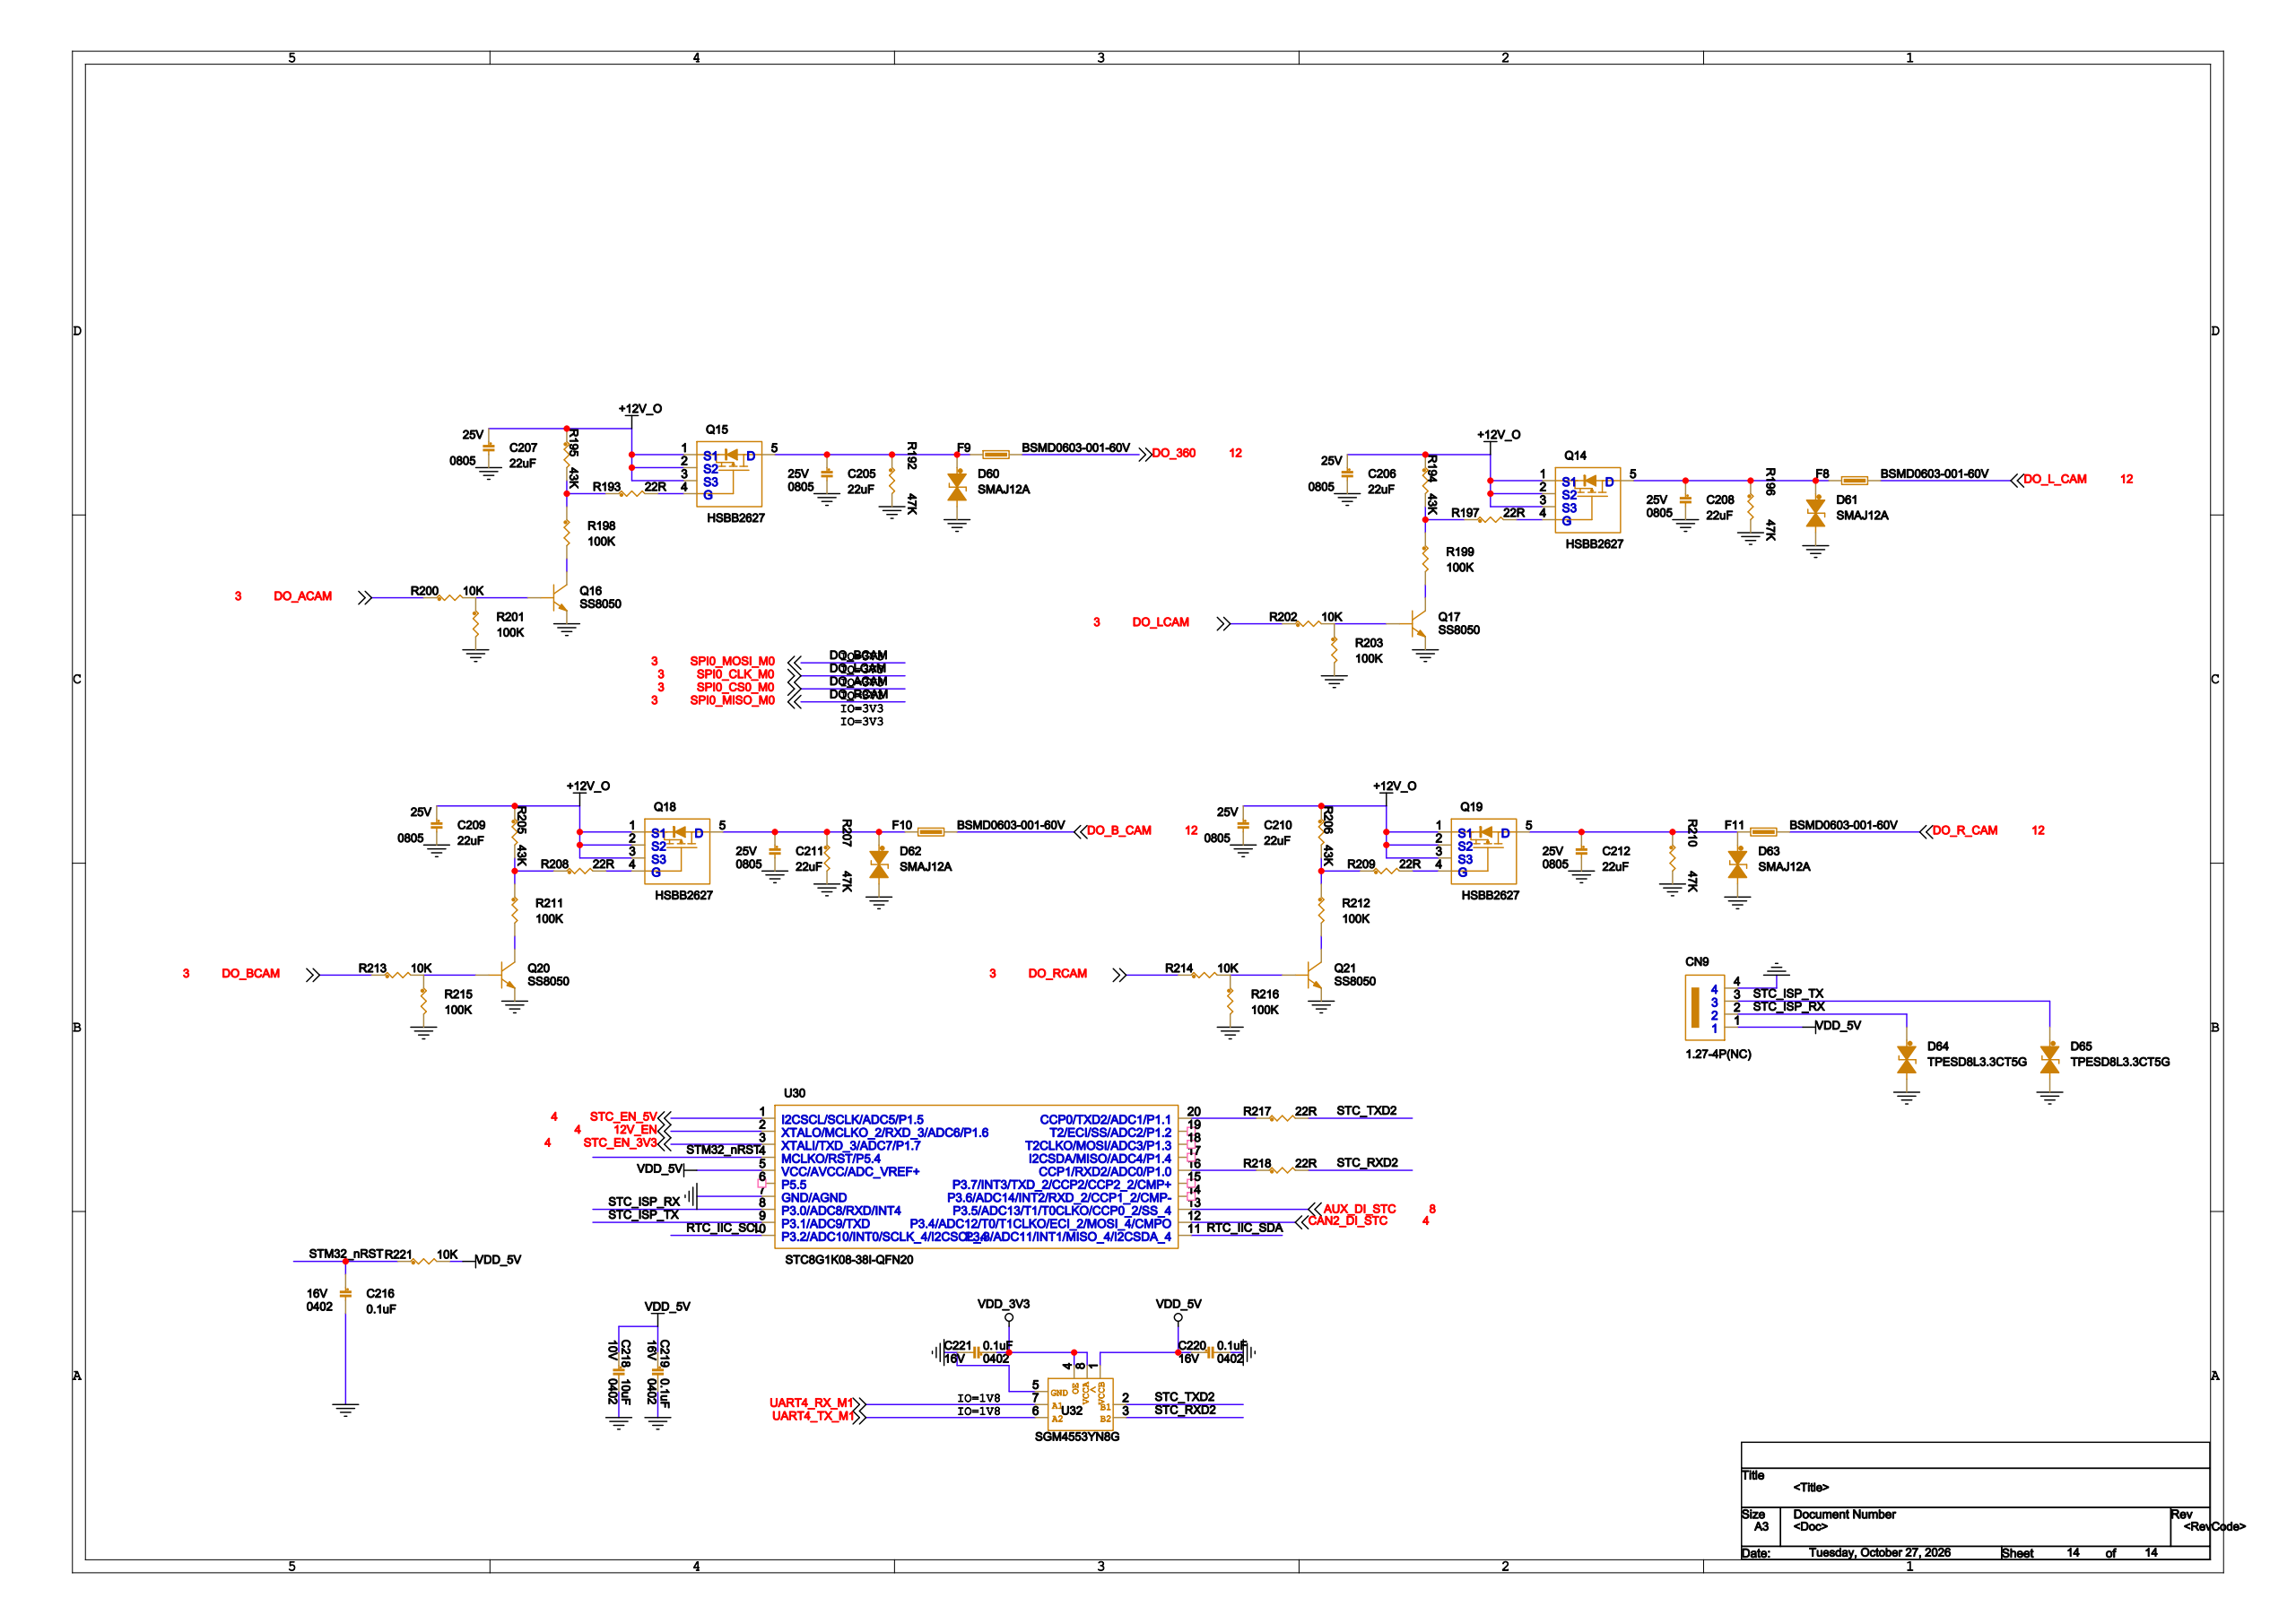Circuit board | Cadence Allegro | 669 parts | 581 nets | one sheet of the schematic
Parts on this sheet (reference | value | footprint):
C205 | 22uF | C0805
C206 | 22uF | C0805
C207 | 22uF | C0805
C208 | 22uF | C0805
C209 | 22uF | C0805
C210 | 22uF | C0805
C211 | 22uF | C0805
C212 | 22uF | C0805
C216 | 0.1uF | C0402
C218 | 10uF | C0402
C219 | 0.1uF | C0402
C220 | 0.1uF | C0402
C221 | 0.1uF | C0402
CN9 | 1.27-4P(NC) | SIP4_1P27
D60 | SMAJ12A | SMA
D61 | SMAJ12A | SMA
D62 | SMAJ12A | SMA
D63 | SMAJ12A | SMA
D64 | TPESD8L3.3CT5G | DFN1006_2L
D65 | TPESD8L3.3CT5G | DFN1006_2L
F8 | BSMD0603-001-60V | R0603
F9 | BSMD0603-001-60V | R0603
F10 | BSMD0603-001-60V | R0603
F11 | BSMD0603-001-60V | R0603
Q14 | HSBB2627 | DFN3X3
Q15 | HSBB2627 | DFN3X3
Q16 | SS8050 | SOT-23
Q17 | SS8050 | SOT-23
Q18 | HSBB2627 | DFN3X3
Q19 | HSBB2627 | DFN3X3
Q20 | SS8050 | SOT-23
Q21 | SS8050 | SOT-23
R192 | 47K | R0805
R193 | 22R | R0402
R194 | 43K | R0402
R195 | 43K | R0402
R196 | 47K | R0805
R197 | 22R | R0402
R198 | 100K | R0402
R199 | 100K | R0402
R200 | 10K | R0402
R201 | 100K | R0402
R202 | 10K | R0402
R203 | 100K | R0402
R205 | 43K | R0402
R206 | 43K | R0402
R207 | 47K | R0805
R208 | 22R | R0402
R209 | 22R | R0402
R210 | 47K | R0805
R211 | 100K | R0402
R212 | 100K | R0402
R213 | 10K | R0402
R214 | 10K | R0402
R215 | 100K | R0402
R216 | 100K | R0402
R217 | 22R | R0402
R218 | 22R | R0402
R221 | 10K | R0402
U30 | STC8G1K08-38I-QFN20 | QFN20_3X3
U32 | SGM4553YN8G | SOT23_8
Nets of these parts (net: part-pin ...):
GND: C205-2 C206-2 C207-2 C208-2 C209-2 C210-2 C211-2 C212-2 C216-2 C218-2 C219-2 C220-2 C221-2 CN9-4 D60-1 D61-1 D62-1 D63-1 D64-1 D65-1 Q16-2 Q17-2 Q20-2 Q21-2 R192-2 R196-2 R201-2 R203-2 R207-2 R210-2 R215-2 R216-2 U30-7 U30-21 U32-5
VDD_5V: C218-1 C219-1 C220-1 CN9-1 R221-2 U30-5 U32-1
STC_EN_3V3: U30-3
CAN2_DI_STC: U30-12
VCC3V3_SYS: C221-1 U32-4 U32-8
+12V_O: C206-1 C207-1 C209-1 C210-1 Q14-1 Q14-2 Q14-3 Q15-1 Q15-2 Q15-3 Q18-1 Q18-2 Q18-3 Q19-1 Q19-2 Q19-3 R194-1 R195-1 R205-1 R206-1
AUX_DI_STC: U30-13
N84715102: C208-1 D61-2 F8-1 Q14-5 R196-1
N84715168: Q14-4 R197-2
N84714976: C205-1 D60-2 F9-1 Q15-5 R192-1
N84715050: Q15-4 R193-2
N84714325: C211-1 D62-2 F10-1 Q18-5 R207-1
N84714391: Q18-4 R208-2
N84714451: C212-1 D63-2 F11-1 Q19-5 R210-1
N84714525: Q19-4 R209-2
STC_ISP_RX: CN9-2 D64-2 U30-8
STC_ISP_TX: CN9-3 D65-2 U30-9
N84699712: R217-1 U30-20
N84699715: R218-1 U30-16
STC_EN_5V: U30-1
STM32_NRST: C216-1 R221-1 U30-4
RTC_IIC_SCL: U30-10
RTC_IIC_SDA: U30-11
12V_EN: U30-2
DO_B_CAM: F10-2
DO_R_CAM: F11-2
DO_L_CAM: F8-2
DO_360: F9-2
N84715020: Q16-1 R200-2 R201-1
N84715048: Q16-3 R198-2
N84715148: Q17-1 R202-2 R203-1
N84715166: Q17-3 R199-2
N84714379: Q20-1 R213-2 R215-1
N84714389: Q20-3 R211-2
N84714495: Q21-1 R214-2 R216-1
N84714523: Q21-3 R212-2
N84714999: R193-1 R195-2 R198-1
N84715125: R194-2 R197-1 R199-1
N84714348: R205-2 R208-1 R211-1
N84714478: R206-2 R209-1 R212-1
STC_TXD2: R217-2 U32-2
STC_RXD2: R218-2 U32-3
DO_ACAM: R200-1
DO_LCAM: R202-1
DO_BCAM: R213-1
DO_RCAM: R214-1
UART4_RX_M1: U32-7
UART4_TX_M1: U32-6